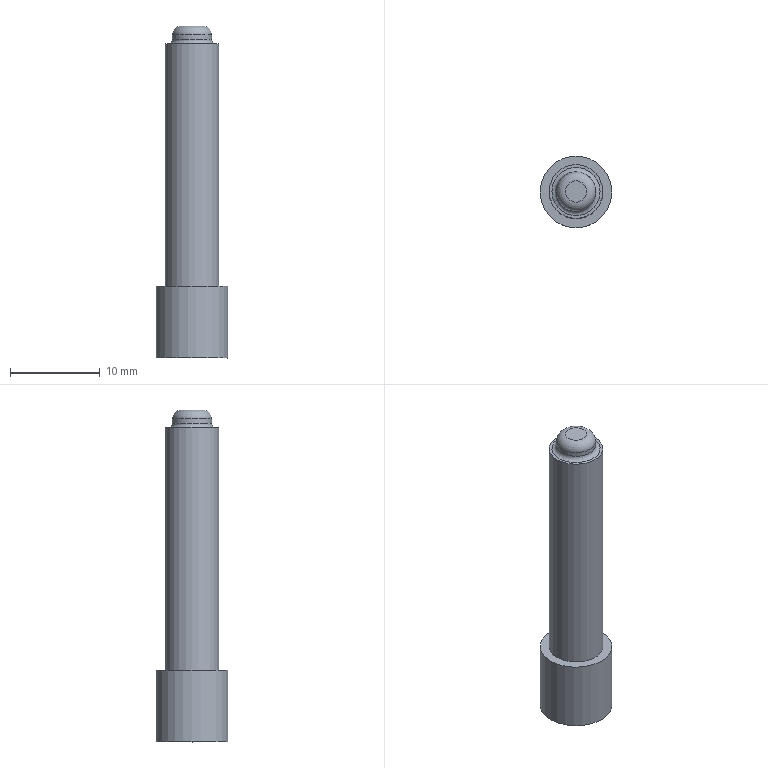Part | NX | features solid 2 | 1 solid | 9 faces | box 8 x 8 x 37 mm | volume 1194 mm3 | plane 4 | cylinder 3 | torus 2 | commonest cylinder face diameters 4.38 x1 6 x1 8 x1
STEP:
#1=CARTESIAN_POINT('',(4187.236,-828.622,858.716));
#2=VERTEX_POINT('',#1);
#3=CARTESIAN_POINT('',(4184.236,-828.622,858.716));
#4=DIRECTION('',(0.,0.,1.));
#5=DIRECTION('',(1.,0.,0.));
#6=AXIS2_PLACEMENT_3D('',#3,#4,#5);
#7=CIRCLE('',#6,3.);
#8=EDGE_CURVE('',#2,#2,#7,.T.);
#9=ORIENTED_EDGE('',*,*,#8,.F.);
#10=EDGE_LOOP('',(#9));
#11=FACE_BOUND('',#10,.T.);
#12=CARTESIAN_POINT('',(4181.236,-828.622,831.716));
#13=VERTEX_POINT('',#12);
#14=CARTESIAN_POINT('',(4184.236,-828.622,831.716));
#15=DIRECTION('',(0.,0.,-1.));
#16=DIRECTION('',(-1.,0.,0.));
#17=AXIS2_PLACEMENT_3D('',#14,#15,#16);
#18=CIRCLE('',#17,3.);
#19=EDGE_CURVE('',#13,#13,#18,.F.);
#20=ORIENTED_EDGE('',*,*,#19,.T.);
#21=EDGE_LOOP('',(#20));
#22=FACE_BOUND('',#21,.T.);
#23=CARTESIAN_POINT('',(4184.236,-828.622,823.716));
#24=DIRECTION('',(0.,0.,1.));
#25=DIRECTION('',(1.,0.,0.));
#26=AXIS2_PLACEMENT_3D('',#23,#24,#25);
#27=CYLINDRICAL_SURFACE('',#26,3.);
#28=ADVANCED_FACE('',(#11,#22),#27,.T.);
#29=CARTESIAN_POINT('',(4186.414,-828.392,859.716));
#30=VERTEX_POINT('',#29);
#31=CARTESIAN_POINT('',(4185.761,-826.733,859.716));
#32=CARTESIAN_POINT('',(4186.65,-828.367,859.716));
#33=CARTESIAN_POINT('',(4186.122,-830.149,859.716));
#34=CARTESIAN_POINT('',(4184.493,-831.035,859.716));
#35=CARTESIAN_POINT('',(4182.711,-830.51,859.716));
#36=CARTESIAN_POINT('',(4181.823,-828.877,859.716));
#37=CARTESIAN_POINT('',(4182.348,-827.098,859.716));
#38=CARTESIAN_POINT('',(4183.978,-826.209,859.716));
#39=CARTESIAN_POINT('',(4185.761,-826.733,859.716));
#40=CARTESIAN_POINT('',(4186.65,-828.367,859.716));
#41=CARTESIAN_POINT('',(4186.122,-830.149,859.716));
#42=B_SPLINE_CURVE_WITH_KNOTS('',3,(#31,#32,#33,#34,#35,#36,#37,#38,#39,#40,#41),.UNSPECIFIED.,.T.,.F.,(1,1,1,1,1,1,1,1,1,1,1,1,1,1,1),(-0.005135,-0.003423,-0.001712,0.,0.001712,0.003423,0.005135,0.006846,0.008558,0.01027,0.01198,0.01369,0.0154,0.01712,0.01883),.UNSPECIFIED.);
#43=EDGE_CURVE('',#30,#30,#42,.T.);
#44=ORIENTED_EDGE('',*,*,#43,.T.);
#45=EDGE_LOOP('',(#44));
#46=FACE_BOUND('',#45,.T.);
#47=CARTESIAN_POINT('',(4186.426,-828.622,859.216));
#48=VERTEX_POINT('',#47);
#49=CARTESIAN_POINT('',(4184.236,-828.622,859.216));
#50=DIRECTION('',(0.,0.,1.));
#51=DIRECTION('',(1.,0.,0.));
#52=AXIS2_PLACEMENT_3D('',#49,#50,#51);
#53=CIRCLE('',#52,2.19);
#54=EDGE_CURVE('',#48,#48,#53,.F.);
#55=ORIENTED_EDGE('',*,*,#54,.F.);
#56=EDGE_LOOP('',(#55));
#57=FACE_BOUND('',#56,.T.);
#58=CARTESIAN_POINT('',(4184.236,-828.622,860.716));
#59=DIRECTION('',(0.,0.,-1.));
#60=DIRECTION('',(-1.,0.,0.));
#61=AXIS2_PLACEMENT_3D('',#58,#59,#60);
#62=CYLINDRICAL_SURFACE('',#61,2.19);
#63=ADVANCED_FACE('',(#46,#57),#62,.T.);
#64=CARTESIAN_POINT('',(4183.046,-828.622,860.716));
#65=VERTEX_POINT('',#64);
#66=CARTESIAN_POINT('',(4184.236,-828.622,860.716));
#67=DIRECTION('',(0.,0.,-1.));
#68=DIRECTION('',(-1.,0.,0.));
#69=AXIS2_PLACEMENT_3D('',#66,#67,#68);
#70=CIRCLE('',#69,1.19);
#71=EDGE_CURVE('',#65,#65,#70,.F.);
#72=ORIENTED_EDGE('',*,*,#71,.T.);
#73=EDGE_LOOP('',(#72));
#74=FACE_BOUND('',#73,.T.);
#75=CARTESIAN_POINT('',(4184.236,-828.622,860.716));
#76=DIRECTION('',(0.,0.,-1.));
#77=DIRECTION('',(-1.,0.,0.));
#78=AXIS2_PLACEMENT_3D('',#75,#76,#77);
#79=PLANE('',#78);
#80=ADVANCED_FACE('',(#74),#79,.F.);
#81=ORIENTED_EDGE('',*,*,#54,.T.);
#82=EDGE_LOOP('',(#81));
#83=FACE_BOUND('',#82,.T.);
#84=CARTESIAN_POINT('',(4186.926,-828.622,858.716));
#85=VERTEX_POINT('',#84);
#86=CARTESIAN_POINT('',(4184.236,-828.622,858.716));
#87=DIRECTION('',(0.,0.,1.));
#88=DIRECTION('',(1.,0.,0.));
#89=AXIS2_PLACEMENT_3D('',#86,#87,#88);
#90=CIRCLE('',#89,2.69);
#91=EDGE_CURVE('',#85,#85,#90,.F.);
#92=ORIENTED_EDGE('',*,*,#91,.F.);
#93=EDGE_LOOP('',(#92));
#94=FACE_BOUND('',#93,.T.);
#95=CARTESIAN_POINT('',(4184.236,-828.622,859.216));
#96=DIRECTION('',(0.,0.,1.));
#97=DIRECTION('',(1.,0.,0.));
#98=AXIS2_PLACEMENT_3D('',#95,#96,#97);
#99=TOROIDAL_SURFACE('',#98,2.69,0.5);
#100=ADVANCED_FACE('',(#83,#94),#99,.F.);
#101=ORIENTED_EDGE('',*,*,#91,.T.);
#102=EDGE_LOOP('',(#101));
#103=FACE_BOUND('',#102,.T.);
#104=ORIENTED_EDGE('',*,*,#8,.T.);
#105=EDGE_LOOP('',(#104));
#106=FACE_BOUND('',#105,.T.);
#107=CARTESIAN_POINT('',(4217.236,-839.122,858.716));
#108=DIRECTION('',(0.,0.,1.));
#109=DIRECTION('',(1.,0.,0.));
#110=AXIS2_PLACEMENT_3D('',#107,#108,#109);
#111=PLANE('',#110);
#112=ADVANCED_FACE('',(#103,#106),#111,.T.);
#113=ORIENTED_EDGE('',*,*,#71,.F.);
#114=EDGE_LOOP('',(#113));
#115=FACE_BOUND('',#114,.T.);
#116=ORIENTED_EDGE('',*,*,#43,.F.);
#117=EDGE_LOOP('',(#116));
#118=FACE_BOUND('',#117,.T.);
#119=CARTESIAN_POINT('',(4184.236,-828.622,859.716));
#120=DIRECTION('',(0.,0.,-1.));
#121=DIRECTION('',(-1.,0.,0.));
#122=AXIS2_PLACEMENT_3D('',#119,#120,#121);
#123=TOROIDAL_SURFACE('',#122,1.19,1.);
#124=ADVANCED_FACE('',(#115,#118),#123,.T.);
#125=CARTESIAN_POINT('',(4180.236,-828.622,823.716));
#126=VERTEX_POINT('',#125);
#127=CARTESIAN_POINT('',(4184.236,-828.622,823.716));
#128=DIRECTION('',(0.,0.,-1.));
#129=DIRECTION('',(-1.,0.,0.));
#130=AXIS2_PLACEMENT_3D('',#127,#128,#129);
#131=CIRCLE('',#130,4.);
#132=EDGE_CURVE('',#126,#126,#131,.F.);
#133=ORIENTED_EDGE('',*,*,#132,.F.);
#134=EDGE_LOOP('',(#133));
#135=FACE_BOUND('',#134,.T.);
#136=CARTESIAN_POINT('',(4184.236,-828.622,823.716));
#137=DIRECTION('',(0.,0.,-1.));
#138=DIRECTION('',(-1.,0.,0.));
#139=AXIS2_PLACEMENT_3D('',#136,#137,#138);
#140=PLANE('',#139);
#141=ADVANCED_FACE('',(#135),#140,.T.);
#142=CARTESIAN_POINT('',(4180.236,-828.622,831.716));
#143=VERTEX_POINT('',#142);
#144=CARTESIAN_POINT('',(4184.236,-828.622,831.716));
#145=DIRECTION('',(0.,0.,-1.));
#146=DIRECTION('',(-1.,0.,0.));
#147=AXIS2_PLACEMENT_3D('',#144,#145,#146);
#148=CIRCLE('',#147,4.);
#149=EDGE_CURVE('',#143,#143,#148,.T.);
#150=ORIENTED_EDGE('',*,*,#149,.T.);
#151=EDGE_LOOP('',(#150));
#152=FACE_BOUND('',#151,.T.);
#153=ORIENTED_EDGE('',*,*,#132,.T.);
#154=EDGE_LOOP('',(#153));
#155=FACE_BOUND('',#154,.T.);
#156=CARTESIAN_POINT('',(4184.236,-828.622,823.716));
#157=DIRECTION('',(0.,0.,1.));
#158=DIRECTION('',(1.,0.,0.));
#159=AXIS2_PLACEMENT_3D('',#156,#157,#158);
#160=CYLINDRICAL_SURFACE('',#159,4.);
#161=ADVANCED_FACE('',(#152,#155),#160,.T.);
#162=ORIENTED_EDGE('',*,*,#19,.F.);
#163=EDGE_LOOP('',(#162));
#164=FACE_BOUND('',#163,.T.);
#165=ORIENTED_EDGE('',*,*,#149,.F.);
#166=EDGE_LOOP('',(#165));
#167=FACE_BOUND('',#166,.T.);
#168=CARTESIAN_POINT('',(4217.236,-877.122,831.716));
#169=DIRECTION('',(0.,0.,-1.));
#170=DIRECTION('',(-1.,0.,0.));
#171=AXIS2_PLACEMENT_3D('',#168,#169,#170);
#172=PLANE('',#171);
#173=ADVANCED_FACE('',(#164,#167),#172,.F.);
#174=CLOSED_SHELL('',(#28,#63,#80,#100,#112,#124,#141,#161,#173));
#175=MANIFOLD_SOLID_BREP('',#174);
#176=(LENGTH_UNIT()NAMED_UNIT(*)SI_UNIT(.MILLI.,.METRE.));
#177=UNCERTAINTY_MEASURE_WITH_UNIT(LENGTH_MEASURE(0.0508),#176,'','');
#178=(NAMED_UNIT(*)PLANE_ANGLE_UNIT()SI_UNIT($,.RADIAN.));
#179=(NAMED_UNIT(*)SI_UNIT($,.STERADIAN.)SOLID_ANGLE_UNIT());
#180=(GEOMETRIC_REPRESENTATION_CONTEXT(3)GLOBAL_UNCERTAINTY_ASSIGNED_CONTEXT((#177))GLOBAL_UNIT_ASSIGNED_CONTEXT((#176,#178,#179))REPRESENTATION_CONTEXT('',''));
#181=ADVANCED_BREP_SHAPE_REPRESENTATION('',(#175),#180);